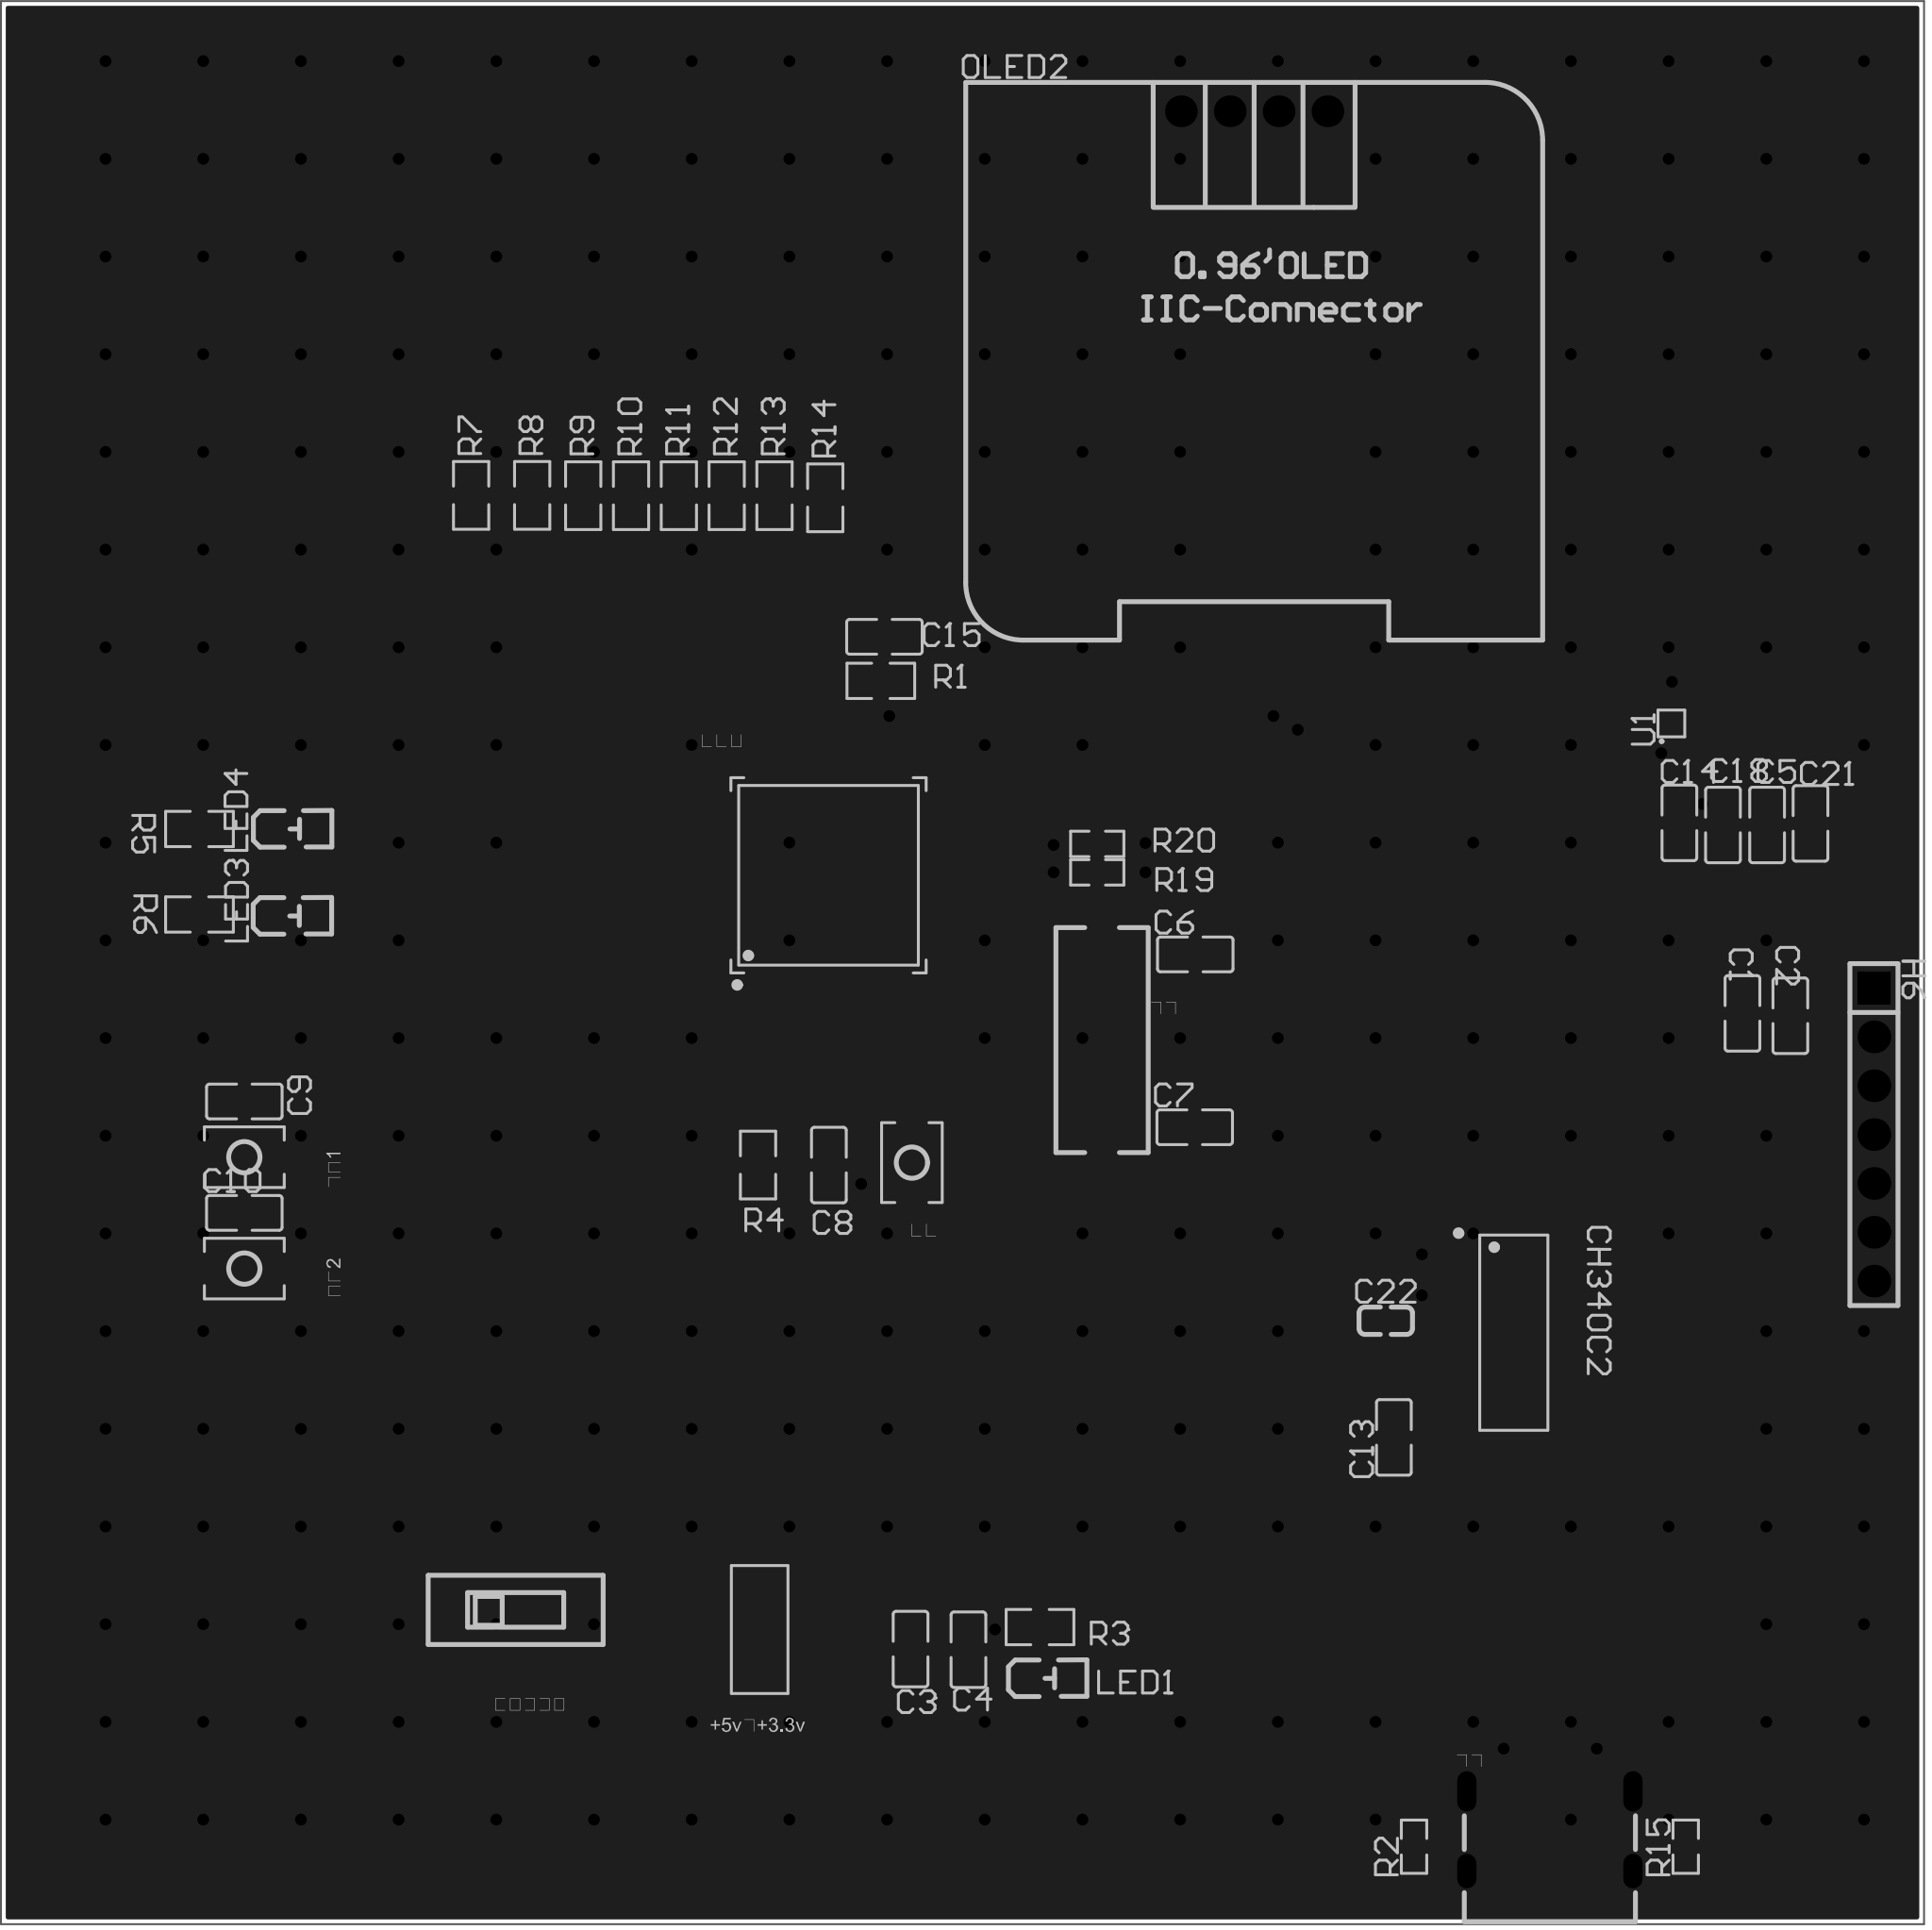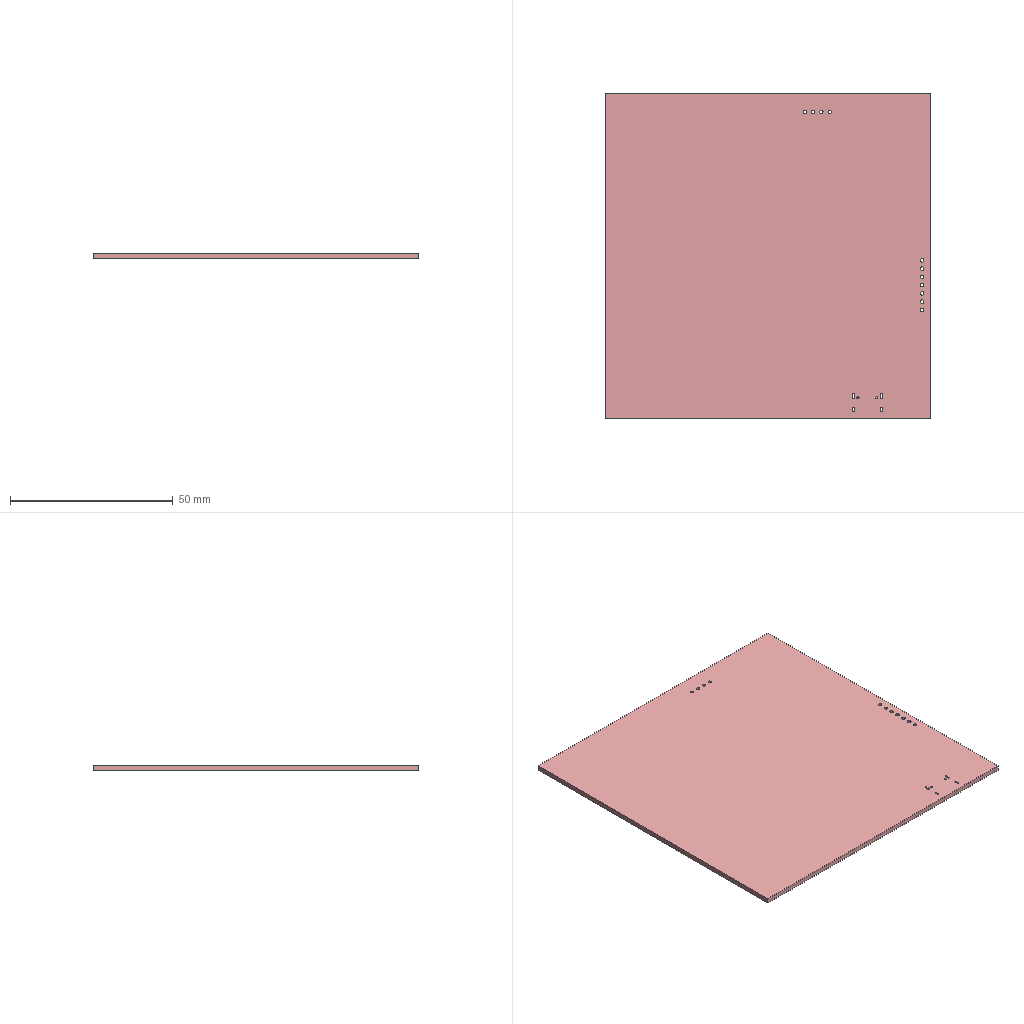Circuit board layout | Altium Designer | box 100 x 100 x 1.6 mm
Layer stack:
# Altium Designer layer stack of  (unit mm; dielectric type: 0 none, 1 core, 2 prepreg, 3 surface material)
index,name,kind,layer,copper_thickness_mm,dielectric_type,dielectric_thickness_mm,dielectric_material,dielectric_constant
0,Top Paste Mask Layer,other,,,,,,
1,Top Silkscreen Layer,other,,,,,,
2,Top Solder Mask Layer,dielectric,,,3,0.01,,3.3
3,Top Layer,copper,Top Layer,0.035,,,,
4,Dielectric1,dielectric,,,3,1.51,FR4,4.5
5,Bottom Layer,copper,Bottom Layer,0.035,,,,
6,Bottom Solder Mask Layer,dielectric,,,3,0.01,,3.3
7,Bottom Silkscreen Layer,other,,,,,,
8,Bottom Paste Mask Layer,other,,,,,,
# drill layer pairs: low layer,high layer
drill_pair,Top Layer,Bottom Layer
Part placement:
Designator,Comment,Layer,Footprint,Center-X(mm),Center-Y(mm),Rotation
C6,22PF,TopLayer,C0805,148.996,139.903,0
C7,22PF,TopLayer,C0805,148.968,130.916,0
晶振,12MHz,TopLayer,CRYSTAL-SMD_L11.4-W4.7-LS12.7,144.15,135.447,270
单片机,STC89C52RC-40I-LQFP44,TopLayer,LQFP-44_L10.0-W10.0-P0.80-LS12.0-BL,129.926,144.016,0
C2,100nF,TopLayer,C0805,179.941,136.712,270
C1,10UF,TopLayer,C0805,177.45,136.838,270
LED1,,TopLayer,LED_0805,141.381,102.261,0
R3,1K,TopLayer,R0805,140.923,104.923,0
C3,100nF,TopLayer,C0805,134.192,103.78,90
C4,10UF,TopLayer,C0805,137.202,103.747,90
+5v转+3.3v,AMS1117-3.3,TopLayer,SOT-223-3_L6.5-W3.4-P2.30-LS7.0-BR,126.445,104.796,0
单片机开关,SS-3235S-L1,TopLayer,SW-SMD_SS-3235S-LX,113.657,105.817,180
H6,,TopLayer,HDR-TH_7P-P2.54-V-M,184.288,130.533,270
R8,10K,TopLayer,R0805,114.516,163.772,90
R13,10K,TopLayer,R0805,127.117,163.756,90
R12,10K,TopLayer,R0805,124.63,163.756,90
R9,10K,TopLayer,R0805,117.171,163.756,90
R11,10K,TopLayer,R0805,122.144,163.756,90
R10,10K,TopLayer,R0805,119.657,163.756,90
R7,10K,TopLayer,R0805,111.341,163.772,90
R14,10K,TopLayer,R0805,129.756,163.645,90
C9,0.1uf,TopLayer,C0805,99.548,132.254,0
功能1,轻触按键3*4*H,TopLayer,SW-SMD_L4.0-W2.9-LS5.0,99.548,129.358,180
C10,0.1uf,TopLayer,C0805,99.548,126.462,0
功能2,轻触按键3*4*H,TopLayer,SW-SMD_L4.0-W2.9-LS5.0,99.548,123.566,180
复位,轻触按键3*4*H,TopLayer,SW-SMD_L4.0-W2.9-LS5.0,134.262,129.076,270
C8,10UF,TopLayer,C0805,129.944,128.949,90
R4,10K,TopLayer,R0805,126.261,128.949,90
LED4,,TopLayer,LED_0805,102.119,146.429,0
LED3,,TopLayer,LED_0805,102.108,141.905,0
R6,1K,TopLayer,R0805,97.216,141.979,180
R5,1K,TopLayer,R0805,97.216,146.424,180
R20,4.7K,TopLayer,R0603,143.9,145.648,180
R19,4.7K,TopLayer,R0603,143.9,144.169,180
C5,2.2uF,TopLayer,C0805,178.732,146.633,270
C13,0.1UF,TopLayer,C0805,159.324,114.787,90
C14,10UF,TopLayer,C0805,174.171,146.744,270
C18,0.1UF,TopLayer,C0805,176.437,146.633,90
C21,0.1UF,TopLayer,C0805,180.989,146.715,90
C22,100nF,TopLayer,C0603,158.902,120.853,0
CH340C2,CH340C,TopLayer,SOP-16_L10.0-W3.9-P1.27-LS6.0-BL,165.561,120.233,270
OLED2,0.96OLED_4P_MODULE_JX,TopLayer,0.96OLED_4P,152.06,183.745,0
C15,0.1uF,TopLayer,C0805,132.833,156.419,180
R1,1K,TopLayer,R0805,132.646,154.128,180
R2,5.1K,TopLayer,R0603,160.373,93.504,90
R15,5.1K,TopLayer,R0603,174.5,93.504,90
U1,BMM350,TopLayer,WLCSP-9_L1.3-W1.3-R3-C3-P0.40-TL,173.755,151.913,90
电源,Type-C,TopLayer,USB-C-SMD_TYPE-C16PIN,167.437,94.597,0
Pad and via stacks:
# Altium Designer via and pad stacks of  (unit mm). Each distinct definition once, with the count of objects using it.
# via: kind,start_layer,end_layer,hole_mm,diameter_mm,mode(0 simple;1 top-mid-bottom;2 full stack),diameter_per_layer,count,example_net
# pad: kind,layer,hole_mm,hole_type(0 round;1 square;2 slot),plating,top_size,top_shape(1 round;2 rect;3 octagon;9 rounded rect),mid_size,bottom_size,mode,footprint,size_per_layer,count,example
pad,Top Layer,0,0,plated,1.41x1.35,2,1.41x1.35,1.41x1.35,0,C0805,,30,C6.2
pad,Top Layer,0,0,plated,5.5x1.4,2,5.5x1.4,5.5x1.4,0,CRYSTAL-SMD_L11.4-W4.7-LS12.7,,2,\u6676\u632F.2
pad,Top Layer,0,0,plated,0.42x1.67,1,0.42x1.67,0.42x1.67,0,LQFP-44_L10.0-W10.0-P0.80-LS12.0-BL,,22,\u5355\u7247\u673A.1
pad,Top Layer,0,0,plated,1.67x0.42,1,1.67x0.42,1.67x0.42,0,LQFP-44_L10.0-W10.0-P0.80-LS12.0-BL,,22,\u5355\u7247\u673A.12
pad,Top Layer,0,0,plated,1x1.25,2,1x1.25,1x1.25,0,LED_0805,,6,LED1.2
pad,Top Layer,0,0,plated,1.133x1.377,2,1.133x1.377,1.133x1.377,0,R0805,,26,R3.2
pad,Top Layer,0,0,plated,2.5x1.1,2,2.5x1.1,2.5x1.1,0,SOT-223-3_L6.5-W3.4-P2.30-LS7.0-BR,,3,+5v\u8F6C+3.3v.1
pad,Top Layer,0,0,plated,2.34x3.6,2,2.34x3.6,2.34x3.6,0,SOT-223-3_L6.5-W3.4-P2.30-LS7.0-BR,,1,+5v\u8F6C+3.3v.4
pad,Top Layer,0,0,plated,0.7x1.8,2,0.7x1.8,0.7x1.8,0,SW-SMD_SS-3235S-LX,,6,\u5355\u7247\u673A\u5F00\u5173.1
pad,Top Layer,0,0,plated,1.53x1.36,2,1.53x1.36,1.53x1.36,0,SW-SMD_L4.0-W2.9-LS5.0,,6,\u529F\u80FD1.1
pad,Top Layer,0,0,plated,0.8065x0.864,2,0.8065x0.864,0.8065x0.864,0,R0603,,8,R20.2
pad,Top Layer,0,0,plated,0.8x0.9,2,0.8x0.9,0.8x0.9,0,C0603,,2,C22.2
pad,Top Layer,0,0,plated,0.56x1.745,1,0.56x1.745,0.56x1.745,0,SOP-16_L10.0-W3.9-P1.27-LS6.0-BL,,16,CH340C2.1
pad,Top Layer,0,0,plated,0.2x0.2,1,0.2x0.2,0.2x0.2,0,WLCSP-9_L1.3-W1.3-R3-C3-P0.40-TL,,9,U1.A1
pad,Top Layer,0,0,plated,0.6x1.15,2,0.6x1.15,0.6x1.15,0,USB-C-SMD_TYPE-C16PIN,,4,\u7535\u6E90.A1B12
pad,Top Layer,0,0,plated,0.3x1.15,2,0.3x1.15,0.3x1.15,0,USB-C-SMD_TYPE-C16PIN,,8,\u7535\u6E90.B5
pad,Multi-Layer,1.1,0,plated,1.7x1.7,2,1.7x1.7,1.7x1.7,0,HDR-TH_7P-P2.54-V-M,,1,H6.1
pad,Multi-Layer,1.1,0,plated,1.7x1.7,1,1.7x1.7,1.7x1.7,0,HDR-TH_7P-P2.54-V-M,,6,H6.2
pad,Multi-Layer,1,0,plated,1.65x1.65,1,1.65x1.65,1.65x1.65,0,0.96OLED_4P,,4,OLED2.4
pad,Multi-Layer,0.6,2,plated,1x1.8,1,1x1.8,1x1.8,0,USB-C-SMD_TYPE-C16PIN,,2,\u7535\u6E90.4
pad,Multi-Layer,0.6,2,plated,1x2.1,1,1x2.1,1x2.1,0,USB-C-SMD_TYPE-C16PIN,,2,\u7535\u6E90.2
via,Top Layer,Bottom Layer,0.3048,0.61,0,,307,P3.1
Copper pours:
name,layer,net,type(0 solid;1 hatched;2 none)
Bottom Layer-GND,Bottom Layer,GND,0
Top Layer-GND,Top Layer,GND,0